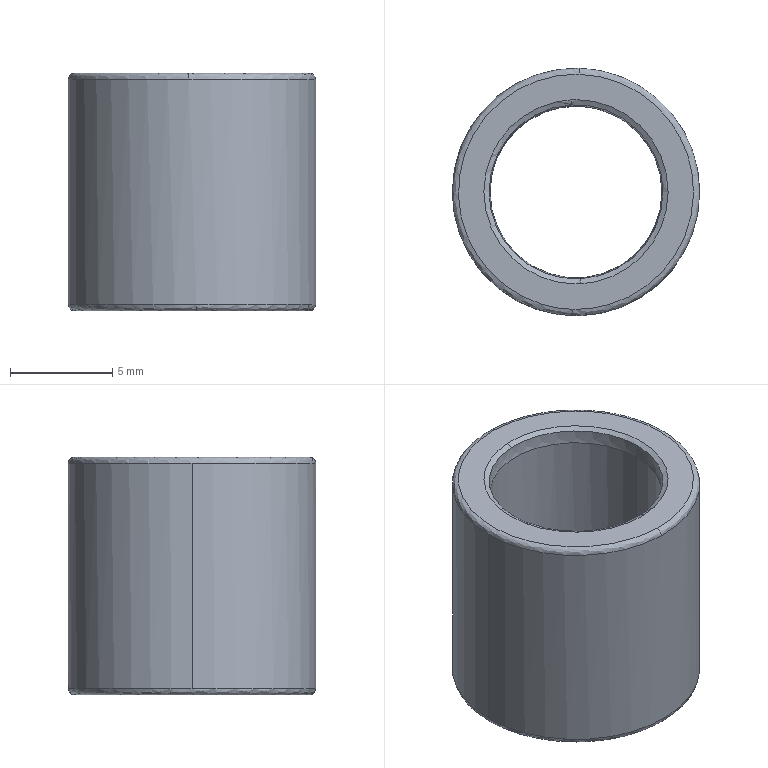Part | STEP file | 12b-1_03 | 1 solid | 16 faces | box 12.07 x 12.07 x 11.6 mm | volume 689.728 mm3 | spline 10 | cylinder 4 | plane 2 | commonest cylinder face diameters 8.39 x2 12.07 x2